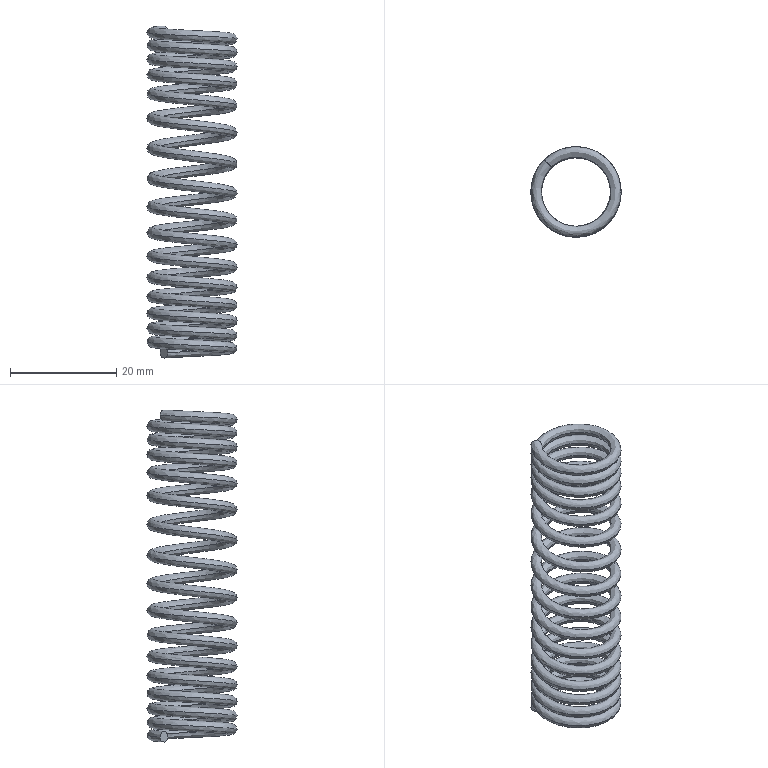Part | STEP file | 2  spring | 1 solid | 4 faces | box 17 x 17 x 62.598 mm | volume 2374 mm3 | spline 2 | plane 2